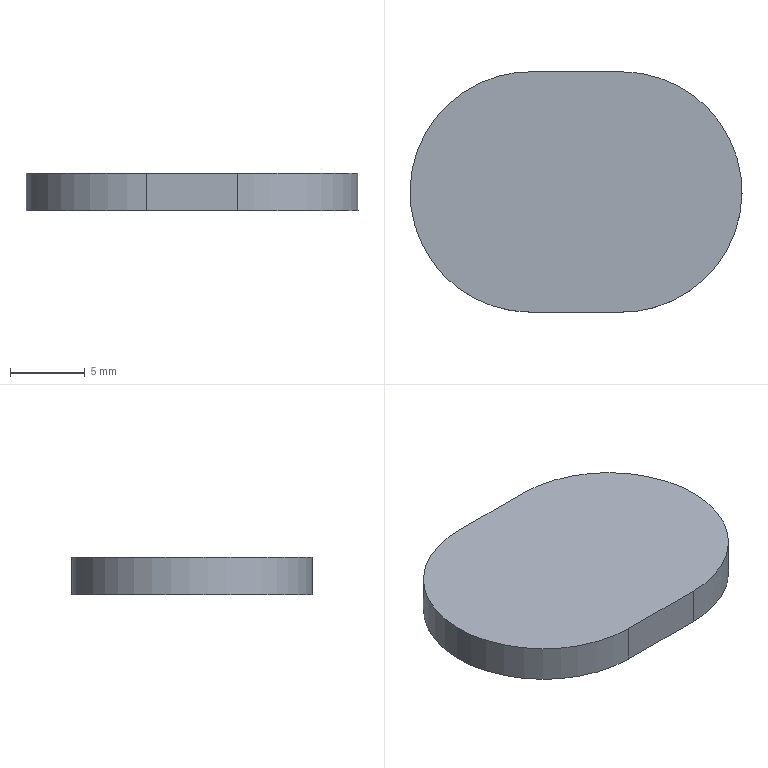Part | STEP file | lll_id1310_x_t | 1 solid | 6 faces | box 22.2 x 16.07 x 2.5 mm | volume 752.765 mm3 | plane 4 | spline 2
STEP:
#1=CARTESIAN_POINT('',(3199.935,163.535,2.5));
#2=VERTEX_POINT('',#1);
#3=CARTESIAN_POINT('',(3206.065,163.535,2.5));
#4=VERTEX_POINT('',#3);
#5=CARTESIAN_POINT('',(3214.,163.535,2.5));
#6=DIRECTION('',(1.,0.,0.000000008));
#7=VECTOR('',#6,1.);
#8=LINE('',#5,#7);
#9=EDGE_CURVE('',#2,#4,#8,.T.);
#10=ORIENTED_EDGE('',*,*,#9,.T.);
#11=CARTESIAN_POINT('',(3206.065,163.535,0.00001609));
#12=VERTEX_POINT('',#11);
#13=CARTESIAN_POINT('',(3206.065,163.535,0.0000161));
#14=DIRECTION('',(-0.000000008,0.,1.));
#15=VECTOR('',#14,1.);
#16=LINE('',#13,#15);
#17=EDGE_CURVE('',#12,#4,#16,.T.);
#18=ORIENTED_EDGE('',*,*,#17,.F.);
#19=CARTESIAN_POINT('',(3199.935,163.535,0.00001605));
#20=VERTEX_POINT('',#19);
#21=CARTESIAN_POINT('',(3214.,163.535,0.00001615));
#22=DIRECTION('',(1.,0.,0.000000008));
#23=VECTOR('',#22,1.);
#24=LINE('',#21,#23);
#25=EDGE_CURVE('',#20,#12,#24,.T.);
#26=ORIENTED_EDGE('',*,*,#25,.F.);
#27=CARTESIAN_POINT('',(3199.935,163.535,0.00001605));
#28=DIRECTION('',(-0.000000008,0.,1.));
#29=VECTOR('',#28,1.);
#30=LINE('',#27,#29);
#31=EDGE_CURVE('',#20,#2,#30,.T.);
#32=ORIENTED_EDGE('',*,*,#31,.T.);
#33=EDGE_LOOP('',(#10,#18,#26,#32));
#34=FACE_OUTER_BOUND('',#33,.T.);
#35=CARTESIAN_POINT('',(3200.,163.535,0.00001605));
#36=DIRECTION('',(0.,-1.,0.));
#37=DIRECTION('',(-0.000000008,0.,1.));
#38=AXIS2_PLACEMENT_3D('',#35,#36,#37);
#39=PLANE('',#38);
#40=ADVANCED_FACE('',(#34),#39,.F.);
#41=CARTESIAN_POINT('',(3206.065,147.465,2.5));
#42=VERTEX_POINT('',#41);
#43=CARTESIAN_POINT('',(3206.065,163.535,2.5));
#44=CARTESIAN_POINT('',(3208.16,163.535,2.5));
#45=CARTESIAN_POINT('',(3210.259,162.67,2.5));
#46=CARTESIAN_POINT('',(3213.235,159.694,2.5));
#47=CARTESIAN_POINT('',(3214.1,157.604,2.5));
#48=CARTESIAN_POINT('',(3214.1,153.396,2.5));
#49=CARTESIAN_POINT('',(3213.235,151.306,2.5));
#50=CARTESIAN_POINT('',(3210.259,148.331,2.5));
#51=CARTESIAN_POINT('',(3208.16,147.465,2.5));
#52=CARTESIAN_POINT('',(3206.065,147.465,2.5));
#53=B_SPLINE_CURVE_WITH_KNOTS('',3,(#43,#44,#45,#46,#47,#48,#49,#50,#51,#52),.UNSPECIFIED.,.F.,.F.,(4,2,2,2,4),(0.,0.25,0.5,0.75,1.),.UNSPECIFIED.);
#54=EDGE_CURVE('',#4,#42,#53,.T.);
#55=ORIENTED_EDGE('',*,*,#54,.T.);
#56=CARTESIAN_POINT('',(3206.065,147.465,0.0000161));
#57=VERTEX_POINT('',#56);
#58=CARTESIAN_POINT('',(3206.065,147.465,0.0000161));
#59=DIRECTION('',(-0.000000008,0.,1.));
#60=VECTOR('',#59,1.);
#61=LINE('',#58,#60);
#62=EDGE_CURVE('',#57,#42,#61,.T.);
#63=ORIENTED_EDGE('',*,*,#62,.F.);
#64=CARTESIAN_POINT('',(3206.065,163.535,0.0000161));
#65=CARTESIAN_POINT('',(3208.16,163.535,0.00001611));
#66=CARTESIAN_POINT('',(3210.259,162.67,0.00001613));
#67=CARTESIAN_POINT('',(3213.235,159.694,0.00001615));
#68=CARTESIAN_POINT('',(3214.1,157.604,0.00001616));
#69=CARTESIAN_POINT('',(3214.1,153.396,0.00001616));
#70=CARTESIAN_POINT('',(3213.235,151.306,0.00001615));
#71=CARTESIAN_POINT('',(3210.259,148.331,0.00001613));
#72=CARTESIAN_POINT('',(3208.16,147.465,0.00001611));
#73=CARTESIAN_POINT('',(3206.065,147.465,0.0000161));
#74=B_SPLINE_CURVE_WITH_KNOTS('',3,(#64,#65,#66,#67,#68,#69,#70,#71,#72,#73),.UNSPECIFIED.,.F.,.F.,(4,2,2,2,4),(0.,0.25,0.5,0.75,1.),.UNSPECIFIED.);
#75=EDGE_CURVE('',#12,#57,#74,.T.);
#76=ORIENTED_EDGE('',*,*,#75,.F.);
#77=ORIENTED_EDGE('',*,*,#17,.T.);
#78=EDGE_LOOP('',(#55,#63,#76,#77));
#79=FACE_OUTER_BOUND('',#78,.T.);
#80=CARTESIAN_POINT('',(3206.065,147.465,0.00001609));
#81=CARTESIAN_POINT('',(3206.065,147.465,2.5));
#82=CARTESIAN_POINT('',(3208.16,147.465,0.00001611));
#83=CARTESIAN_POINT('',(3208.16,147.465,2.5));
#84=CARTESIAN_POINT('',(3210.259,148.331,0.00001613));
#85=CARTESIAN_POINT('',(3210.259,148.331,2.5));
#86=CARTESIAN_POINT('',(3213.235,151.306,0.00001615));
#87=CARTESIAN_POINT('',(3213.235,151.306,2.5));
#88=CARTESIAN_POINT('',(3214.1,153.396,0.00001616));
#89=CARTESIAN_POINT('',(3214.1,153.396,2.5));
#90=CARTESIAN_POINT('',(3214.1,157.604,0.00001616));
#91=CARTESIAN_POINT('',(3214.1,157.604,2.5));
#92=CARTESIAN_POINT('',(3213.235,159.694,0.00001615));
#93=CARTESIAN_POINT('',(3213.235,159.694,2.5));
#94=CARTESIAN_POINT('',(3210.259,162.67,0.00001613));
#95=CARTESIAN_POINT('',(3210.259,162.67,2.5));
#96=CARTESIAN_POINT('',(3208.16,163.535,0.00001611));
#97=CARTESIAN_POINT('',(3208.16,163.535,2.5));
#98=CARTESIAN_POINT('',(3206.065,163.535,0.00001609));
#99=CARTESIAN_POINT('',(3206.065,163.535,2.5));
#100=B_SPLINE_SURFACE_WITH_KNOTS('',3,1,((#80,#81),(#82,#83),(#84,#85),(#86,#87),(#88,#89),(#90,#91),(#92,#93),(#94,#95),(#96,#97),(#98,#99)),.UNSPECIFIED.,.F.,.F.,.F.,(4,2,2,2,4),(2,2),(0.,0.25,0.5,0.75,1.),(0.,1.),.UNSPECIFIED.);
#101=ADVANCED_FACE('',(#79),#100,.T.);
#102=CARTESIAN_POINT('',(3199.935,147.465,2.5));
#103=VERTEX_POINT('',#102);
#104=CARTESIAN_POINT('',(3214.,147.465,2.5));
#105=DIRECTION('',(-1.,0.,-0.000000008));
#106=VECTOR('',#105,1.);
#107=LINE('',#104,#106);
#108=EDGE_CURVE('',#42,#103,#107,.T.);
#109=ORIENTED_EDGE('',*,*,#108,.T.);
#110=CARTESIAN_POINT('',(3199.935,147.465,0.00001605));
#111=VERTEX_POINT('',#110);
#112=CARTESIAN_POINT('',(3199.935,147.465,0.00001605));
#113=DIRECTION('',(-0.000000008,0.,1.));
#114=VECTOR('',#113,1.);
#115=LINE('',#112,#114);
#116=EDGE_CURVE('',#111,#103,#115,.T.);
#117=ORIENTED_EDGE('',*,*,#116,.F.);
#118=CARTESIAN_POINT('',(3214.,147.465,0.00001616));
#119=DIRECTION('',(-1.,0.,-0.000000008));
#120=VECTOR('',#119,1.);
#121=LINE('',#118,#120);
#122=EDGE_CURVE('',#57,#111,#121,.T.);
#123=ORIENTED_EDGE('',*,*,#122,.F.);
#124=ORIENTED_EDGE('',*,*,#62,.T.);
#125=EDGE_LOOP('',(#109,#117,#123,#124));
#126=FACE_OUTER_BOUND('',#125,.T.);
#127=CARTESIAN_POINT('',(3206.,147.465,0.00001609));
#128=DIRECTION('',(0.,1.,0.));
#129=DIRECTION('',(0.000000008,0.,-1.));
#130=AXIS2_PLACEMENT_3D('',#127,#128,#129);
#131=PLANE('',#130);
#132=ADVANCED_FACE('',(#126),#131,.F.);
#133=CARTESIAN_POINT('',(3199.935,147.465,2.5));
#134=CARTESIAN_POINT('',(3197.841,147.465,2.5));
#135=CARTESIAN_POINT('',(3195.741,148.331,2.5));
#136=CARTESIAN_POINT('',(3192.766,151.306,2.5));
#137=CARTESIAN_POINT('',(3191.9,153.396,2.5));
#138=CARTESIAN_POINT('',(3191.9,157.604,2.5));
#139=CARTESIAN_POINT('',(3192.766,159.694,2.5));
#140=CARTESIAN_POINT('',(3195.741,162.67,2.5));
#141=CARTESIAN_POINT('',(3197.841,163.535,2.5));
#142=CARTESIAN_POINT('',(3199.935,163.535,2.5));
#143=B_SPLINE_CURVE_WITH_KNOTS('',3,(#133,#134,#135,#136,#137,#138,#139,#140,#141,#142),.UNSPECIFIED.,.F.,.F.,(4,2,2,2,4),(0.,0.25,0.5,0.75,1.),.UNSPECIFIED.);
#144=EDGE_CURVE('',#103,#2,#143,.T.);
#145=ORIENTED_EDGE('',*,*,#144,.T.);
#146=ORIENTED_EDGE('',*,*,#31,.F.);
#147=CARTESIAN_POINT('',(3199.935,147.465,0.00001605));
#148=CARTESIAN_POINT('',(3197.841,147.465,0.00001603));
#149=CARTESIAN_POINT('',(3195.741,148.331,0.00001602));
#150=CARTESIAN_POINT('',(3192.766,151.306,0.00001599));
#151=CARTESIAN_POINT('',(3191.9,153.396,0.00001599));
#152=CARTESIAN_POINT('',(3191.9,157.604,0.00001599));
#153=CARTESIAN_POINT('',(3192.766,159.694,0.00001599));
#154=CARTESIAN_POINT('',(3195.741,162.67,0.00001602));
#155=CARTESIAN_POINT('',(3197.841,163.535,0.00001603));
#156=CARTESIAN_POINT('',(3199.935,163.535,0.00001605));
#157=B_SPLINE_CURVE_WITH_KNOTS('',3,(#147,#148,#149,#150,#151,#152,#153,#154,#155,#156),.UNSPECIFIED.,.F.,.F.,(4,2,2,2,4),(0.,0.25,0.5,0.75,1.),.UNSPECIFIED.);
#158=EDGE_CURVE('',#111,#20,#157,.T.);
#159=ORIENTED_EDGE('',*,*,#158,.F.);
#160=ORIENTED_EDGE('',*,*,#116,.T.);
#161=EDGE_LOOP('',(#145,#146,#159,#160));
#162=FACE_OUTER_BOUND('',#161,.T.);
#163=CARTESIAN_POINT('',(3199.935,163.535,0.00001605));
#164=CARTESIAN_POINT('',(3199.935,163.535,2.5));
#165=CARTESIAN_POINT('',(3197.841,163.535,0.00001603));
#166=CARTESIAN_POINT('',(3197.841,163.535,2.5));
#167=CARTESIAN_POINT('',(3195.741,162.67,0.00001602));
#168=CARTESIAN_POINT('',(3195.741,162.67,2.5));
#169=CARTESIAN_POINT('',(3192.766,159.694,0.00001599));
#170=CARTESIAN_POINT('',(3192.766,159.694,2.5));
#171=CARTESIAN_POINT('',(3191.9,157.604,0.00001599));
#172=CARTESIAN_POINT('',(3191.9,157.604,2.5));
#173=CARTESIAN_POINT('',(3191.9,153.396,0.00001599));
#174=CARTESIAN_POINT('',(3191.9,153.396,2.5));
#175=CARTESIAN_POINT('',(3192.766,151.306,0.00001599));
#176=CARTESIAN_POINT('',(3192.766,151.306,2.5));
#177=CARTESIAN_POINT('',(3195.741,148.331,0.00001602));
#178=CARTESIAN_POINT('',(3195.741,148.331,2.5));
#179=CARTESIAN_POINT('',(3197.841,147.465,0.00001603));
#180=CARTESIAN_POINT('',(3197.841,147.465,2.5));
#181=CARTESIAN_POINT('',(3199.935,147.465,0.00001605));
#182=CARTESIAN_POINT('',(3199.935,147.465,2.5));
#183=B_SPLINE_SURFACE_WITH_KNOTS('',3,1,((#163,#164),(#165,#166),(#167,#168),(#169,#170),(#171,#172),(#173,#174),(#175,#176),(#177,#178),(#179,#180),(#181,#182)),.UNSPECIFIED.,.F.,.F.,.F.,(4,2,2,2,4),(2,2),(0.,0.25,0.5,0.75,1.),(0.,1.),.UNSPECIFIED.);
#184=ADVANCED_FACE('',(#162),#183,.T.);
#185=ORIENTED_EDGE('',*,*,#25,.T.);
#186=ORIENTED_EDGE('',*,*,#75,.T.);
#187=ORIENTED_EDGE('',*,*,#122,.T.);
#188=ORIENTED_EDGE('',*,*,#158,.T.);
#189=EDGE_LOOP('',(#185,#186,#187,#188));
#190=FACE_OUTER_BOUND('',#189,.T.);
#191=CARTESIAN_POINT('',(3214.,155.5,0.00001616));
#192=DIRECTION('',(-0.000000008,0.,1.));
#193=DIRECTION('',(0.,1.,0.));
#194=AXIS2_PLACEMENT_3D('',#191,#192,#193);
#195=PLANE('',#194);
#196=ADVANCED_FACE('',(#190),#195,.F.);
#197=ORIENTED_EDGE('',*,*,#9,.F.);
#198=ORIENTED_EDGE('',*,*,#144,.F.);
#199=ORIENTED_EDGE('',*,*,#108,.F.);
#200=ORIENTED_EDGE('',*,*,#54,.F.);
#201=EDGE_LOOP('',(#197,#198,#199,#200));
#202=FACE_OUTER_BOUND('',#201,.T.);
#203=CARTESIAN_POINT('',(3214.,155.5,2.5));
#204=DIRECTION('',(-0.000000008,0.,1.));
#205=DIRECTION('',(0.,1.,0.));
#206=AXIS2_PLACEMENT_3D('',#203,#204,#205);
#207=PLANE('',#206);
#208=ADVANCED_FACE('',(#202),#207,.T.);
#209=CLOSED_SHELL('',(#40,#101,#132,#184,#196,#208));
#210=MANIFOLD_SOLID_BREP('',#209);
#211=(LENGTH_UNIT()NAMED_UNIT(*)SI_UNIT(.MILLI.,.METRE.));
#212=UNCERTAINTY_MEASURE_WITH_UNIT(LENGTH_MEASURE(0.00002),#211,'','');
#213=(NAMED_UNIT(*)PLANE_ANGLE_UNIT()SI_UNIT($,.RADIAN.));
#214=PLANE_ANGLE_MEASURE_WITH_UNIT(PLANE_ANGLE_MEASURE(0.01745),#213);
#215=DIMENSIONAL_EXPONENTS(0.,0.,0.,0.,0.,0.,0.);
#216=(CONVERSION_BASED_UNIT('DEGREE',#214)NAMED_UNIT(#215)PLANE_ANGLE_UNIT());
#217=(NAMED_UNIT(*)SI_UNIT($,.STERADIAN.)SOLID_ANGLE_UNIT());
#218=(GEOMETRIC_REPRESENTATION_CONTEXT(3)GLOBAL_UNCERTAINTY_ASSIGNED_CONTEXT((#212))GLOBAL_UNIT_ASSIGNED_CONTEXT((#211,#216,#217))REPRESENTATION_CONTEXT('',''));
#219=ADVANCED_BREP_SHAPE_REPRESENTATION('',(#210),#218);